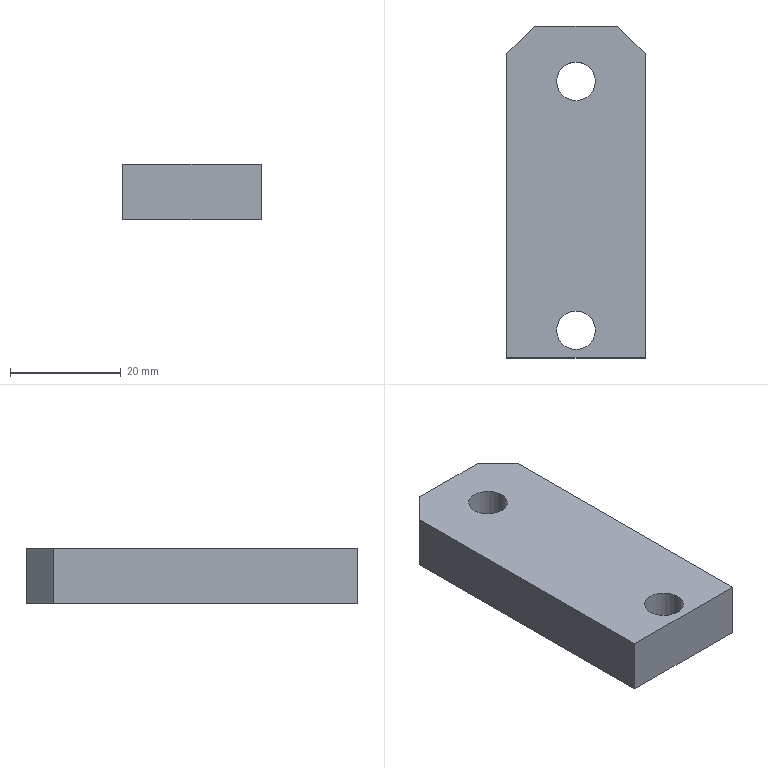Part | SolidWorks | features Chamfer 1, Extrusion 1, ICE 1 | 1 solid | 12 faces | box 25 x 60 x 10 mm | volume 13980 mm3 | plane 8 | cylinder 4 | commonest cylinder face diameters 7 x4
STEP:
#1=CARTESIAN_POINT('',(-3.5,20.,0.));
#2=VERTEX_POINT('',#1);
#3=CARTESIAN_POINT('',(3.5,20.,0.));
#4=VERTEX_POINT('',#3);
#5=CARTESIAN_POINT('',(0.,20.,0.));
#6=DIRECTION('',(0.,0.,1.));
#7=DIRECTION('',(1.,0.,0.));
#8=AXIS2_PLACEMENT_3D('',#5,#6,#7);
#9=CIRCLE('',#8,3.5);
#10=EDGE_CURVE('',#2,#4,#9,.T.);
#11=ORIENTED_EDGE('',*,*,#10,.F.);
#12=CARTESIAN_POINT('',(-3.5,20.,10.));
#13=VERTEX_POINT('',#12);
#14=CARTESIAN_POINT('',(-3.5,20.,0.));
#15=DIRECTION('',(0.,0.,1.));
#16=VECTOR('',#15,1000.);
#17=LINE('',#14,#16);
#18=EDGE_CURVE('',#2,#13,#17,.T.);
#19=ORIENTED_EDGE('',*,*,#18,.T.);
#20=CARTESIAN_POINT('',(3.5,20.,10.));
#21=VERTEX_POINT('',#20);
#22=CARTESIAN_POINT('',(0.,20.,10.));
#23=DIRECTION('',(0.,0.,1.));
#24=DIRECTION('',(1.,0.,0.));
#25=AXIS2_PLACEMENT_3D('',#22,#23,#24);
#26=CIRCLE('',#25,3.5);
#27=EDGE_CURVE('',#13,#21,#26,.T.);
#28=ORIENTED_EDGE('',*,*,#27,.T.);
#29=CARTESIAN_POINT('',(3.5,20.,0.));
#30=DIRECTION('',(0.,0.,1.));
#31=VECTOR('',#30,1000.);
#32=LINE('',#29,#31);
#33=EDGE_CURVE('',#4,#21,#32,.T.);
#34=ORIENTED_EDGE('',*,*,#33,.F.);
#35=EDGE_LOOP('',(#11,#19,#28,#34));
#36=FACE_OUTER_BOUND('',#35,.T.);
#37=CARTESIAN_POINT('',(0.,20.,0.));
#38=DIRECTION('',(0.,0.,1.));
#39=DIRECTION('',(1.,0.,0.));
#40=AXIS2_PLACEMENT_3D('',#37,#38,#39);
#41=CYLINDRICAL_SURFACE('',#40,3.5);
#42=ADVANCED_FACE('',(#36),#41,.F.);
#43=CARTESIAN_POINT('',(-3.5,-25.,0.));
#44=VERTEX_POINT('',#43);
#45=CARTESIAN_POINT('',(3.5,-25.,0.));
#46=VERTEX_POINT('',#45);
#47=CARTESIAN_POINT('',(0.,-25.,0.));
#48=DIRECTION('',(0.,0.,1.));
#49=DIRECTION('',(1.,0.,0.));
#50=AXIS2_PLACEMENT_3D('',#47,#48,#49);
#51=CIRCLE('',#50,3.5);
#52=EDGE_CURVE('',#44,#46,#51,.T.);
#53=ORIENTED_EDGE('',*,*,#52,.F.);
#54=CARTESIAN_POINT('',(-3.5,-25.,10.));
#55=VERTEX_POINT('',#54);
#56=CARTESIAN_POINT('',(-3.5,-25.,0.));
#57=DIRECTION('',(0.,0.,1.));
#58=VECTOR('',#57,1000.);
#59=LINE('',#56,#58);
#60=EDGE_CURVE('',#44,#55,#59,.T.);
#61=ORIENTED_EDGE('',*,*,#60,.T.);
#62=CARTESIAN_POINT('',(3.5,-25.,10.));
#63=VERTEX_POINT('',#62);
#64=CARTESIAN_POINT('',(0.,-25.,10.));
#65=DIRECTION('',(0.,0.,1.));
#66=DIRECTION('',(1.,0.,0.));
#67=AXIS2_PLACEMENT_3D('',#64,#65,#66);
#68=CIRCLE('',#67,3.5);
#69=EDGE_CURVE('',#55,#63,#68,.T.);
#70=ORIENTED_EDGE('',*,*,#69,.T.);
#71=CARTESIAN_POINT('',(3.5,-25.,0.));
#72=DIRECTION('',(0.,0.,1.));
#73=VECTOR('',#72,1000.);
#74=LINE('',#71,#73);
#75=EDGE_CURVE('',#46,#63,#74,.T.);
#76=ORIENTED_EDGE('',*,*,#75,.F.);
#77=EDGE_LOOP('',(#53,#61,#70,#76));
#78=FACE_OUTER_BOUND('',#77,.T.);
#79=CARTESIAN_POINT('',(0.,-25.,0.));
#80=DIRECTION('',(0.,0.,1.));
#81=DIRECTION('',(1.,0.,0.));
#82=AXIS2_PLACEMENT_3D('',#79,#80,#81);
#83=CYLINDRICAL_SURFACE('',#82,3.5);
#84=ADVANCED_FACE('',(#78),#83,.F.);
#85=CARTESIAN_POINT('',(-12.5,25.,10.));
#86=VERTEX_POINT('',#85);
#87=CARTESIAN_POINT('',(-12.5,-30.,10.));
#88=VERTEX_POINT('',#87);
#89=CARTESIAN_POINT('',(-12.5,30.,10.));
#90=DIRECTION('',(0.,-1.,0.));
#91=VECTOR('',#90,1000.);
#92=LINE('',#89,#91);
#93=EDGE_CURVE('',#86,#88,#92,.T.);
#94=ORIENTED_EDGE('',*,*,#93,.F.);
#95=CARTESIAN_POINT('',(-12.5,25.,0.));
#96=VERTEX_POINT('',#95);
#97=CARTESIAN_POINT('',(-12.5,25.,10.));
#98=DIRECTION('',(0.,0.,-1.));
#99=VECTOR('',#98,1000.);
#100=LINE('',#97,#99);
#101=EDGE_CURVE('',#86,#96,#100,.T.);
#102=ORIENTED_EDGE('',*,*,#101,.T.);
#103=CARTESIAN_POINT('',(-12.5,-30.,0.));
#104=VERTEX_POINT('',#103);
#105=CARTESIAN_POINT('',(-12.5,30.,0.));
#106=DIRECTION('',(0.,-1.,0.));
#107=VECTOR('',#106,1000.);
#108=LINE('',#105,#107);
#109=EDGE_CURVE('',#96,#104,#108,.T.);
#110=ORIENTED_EDGE('',*,*,#109,.T.);
#111=CARTESIAN_POINT('',(-12.5,-30.,10.));
#112=DIRECTION('',(0.,0.,-1.));
#113=VECTOR('',#112,1000.);
#114=LINE('',#111,#113);
#115=EDGE_CURVE('',#88,#104,#114,.T.);
#116=ORIENTED_EDGE('',*,*,#115,.F.);
#117=EDGE_LOOP('',(#94,#102,#110,#116));
#118=FACE_OUTER_BOUND('',#117,.T.);
#119=CARTESIAN_POINT('',(-12.5,30.,10.));
#120=DIRECTION('',(1.,0.,0.));
#121=DIRECTION('',(0.,1.,0.));
#122=AXIS2_PLACEMENT_3D('',#119,#120,#121);
#123=PLANE('',#122);
#124=ADVANCED_FACE('',(#118),#123,.F.);
#125=CARTESIAN_POINT('',(12.5,-30.,0.));
#126=VERTEX_POINT('',#125);
#127=CARTESIAN_POINT('',(12.5,-30.,0.));
#128=DIRECTION('',(1.,0.,0.));
#129=VECTOR('',#128,1000.);
#130=LINE('',#127,#129);
#131=EDGE_CURVE('',#104,#126,#130,.T.);
#132=ORIENTED_EDGE('',*,*,#131,.T.);
#133=CARTESIAN_POINT('',(12.5,-30.,10.));
#134=VERTEX_POINT('',#133);
#135=CARTESIAN_POINT('',(12.5,-30.,10.));
#136=DIRECTION('',(0.,0.,-1.));
#137=VECTOR('',#136,1000.);
#138=LINE('',#135,#137);
#139=EDGE_CURVE('',#134,#126,#138,.T.);
#140=ORIENTED_EDGE('',*,*,#139,.F.);
#141=CARTESIAN_POINT('',(12.5,-30.,10.));
#142=DIRECTION('',(1.,0.,0.));
#143=VECTOR('',#142,1000.);
#144=LINE('',#141,#143);
#145=EDGE_CURVE('',#88,#134,#144,.T.);
#146=ORIENTED_EDGE('',*,*,#145,.F.);
#147=ORIENTED_EDGE('',*,*,#115,.T.);
#148=EDGE_LOOP('',(#132,#140,#146,#147));
#149=FACE_OUTER_BOUND('',#148,.T.);
#150=CARTESIAN_POINT('',(12.5,-30.,10.));
#151=DIRECTION('',(0.,1.,0.));
#152=DIRECTION('',(-1.,0.,0.));
#153=AXIS2_PLACEMENT_3D('',#150,#151,#152);
#154=PLANE('',#153);
#155=ADVANCED_FACE('',(#149),#154,.F.);
#156=CARTESIAN_POINT('',(12.5,25.,0.));
#157=VERTEX_POINT('',#156);
#158=CARTESIAN_POINT('',(12.5,30.,0.));
#159=DIRECTION('',(0.,1.,0.));
#160=VECTOR('',#159,1000.);
#161=LINE('',#158,#160);
#162=EDGE_CURVE('',#126,#157,#161,.T.);
#163=ORIENTED_EDGE('',*,*,#162,.T.);
#164=CARTESIAN_POINT('',(12.5,25.,10.));
#165=VERTEX_POINT('',#164);
#166=CARTESIAN_POINT('',(12.5,25.,10.));
#167=DIRECTION('',(0.,0.,1.));
#168=VECTOR('',#167,1000.);
#169=LINE('',#166,#168);
#170=EDGE_CURVE('',#157,#165,#169,.T.);
#171=ORIENTED_EDGE('',*,*,#170,.T.);
#172=CARTESIAN_POINT('',(12.5,30.,10.));
#173=DIRECTION('',(0.,1.,0.));
#174=VECTOR('',#173,1000.);
#175=LINE('',#172,#174);
#176=EDGE_CURVE('',#134,#165,#175,.T.);
#177=ORIENTED_EDGE('',*,*,#176,.F.);
#178=ORIENTED_EDGE('',*,*,#139,.T.);
#179=EDGE_LOOP('',(#163,#171,#177,#178));
#180=FACE_OUTER_BOUND('',#179,.T.);
#181=CARTESIAN_POINT('',(12.5,30.,10.));
#182=DIRECTION('',(-1.,0.,0.));
#183=DIRECTION('',(0.,-1.,0.));
#184=AXIS2_PLACEMENT_3D('',#181,#182,#183);
#185=PLANE('',#184);
#186=ADVANCED_FACE('',(#180),#185,.F.);
#187=CARTESIAN_POINT('',(7.5,30.,10.));
#188=VERTEX_POINT('',#187);
#189=CARTESIAN_POINT('',(-7.5,30.,10.));
#190=VERTEX_POINT('',#189);
#191=CARTESIAN_POINT('',(12.5,30.,10.));
#192=DIRECTION('',(-1.,0.,0.));
#193=VECTOR('',#192,1000.);
#194=LINE('',#191,#193);
#195=EDGE_CURVE('',#188,#190,#194,.T.);
#196=ORIENTED_EDGE('',*,*,#195,.F.);
#197=CARTESIAN_POINT('',(7.5,30.,0.));
#198=VERTEX_POINT('',#197);
#199=CARTESIAN_POINT('',(7.5,30.,10.));
#200=DIRECTION('',(0.,0.,-1.));
#201=VECTOR('',#200,1000.);
#202=LINE('',#199,#201);
#203=EDGE_CURVE('',#188,#198,#202,.T.);
#204=ORIENTED_EDGE('',*,*,#203,.T.);
#205=CARTESIAN_POINT('',(-7.5,30.,0.));
#206=VERTEX_POINT('',#205);
#207=CARTESIAN_POINT('',(12.5,30.,0.));
#208=DIRECTION('',(-1.,0.,0.));
#209=VECTOR('',#208,1000.);
#210=LINE('',#207,#209);
#211=EDGE_CURVE('',#198,#206,#210,.T.);
#212=ORIENTED_EDGE('',*,*,#211,.T.);
#213=CARTESIAN_POINT('',(-7.5,30.,10.));
#214=DIRECTION('',(0.,0.,1.));
#215=VECTOR('',#214,1000.);
#216=LINE('',#213,#215);
#217=EDGE_CURVE('',#206,#190,#216,.T.);
#218=ORIENTED_EDGE('',*,*,#217,.T.);
#219=EDGE_LOOP('',(#196,#204,#212,#218));
#220=FACE_OUTER_BOUND('',#219,.T.);
#221=CARTESIAN_POINT('',(12.5,30.,10.));
#222=DIRECTION('',(0.,-1.,0.));
#223=DIRECTION('',(0.,0.,-1.));
#224=AXIS2_PLACEMENT_3D('',#221,#222,#223);
#225=PLANE('',#224);
#226=ADVANCED_FACE('',(#220),#225,.F.);
#227=CARTESIAN_POINT('',(0.,20.,10.));
#228=DIRECTION('',(0.,0.,1.));
#229=DIRECTION('',(1.,0.,0.));
#230=AXIS2_PLACEMENT_3D('',#227,#228,#229);
#231=CIRCLE('',#230,3.5);
#232=EDGE_CURVE('',#21,#13,#231,.T.);
#233=ORIENTED_EDGE('',*,*,#232,.F.);
#234=ORIENTED_EDGE('',*,*,#27,.F.);
#235=EDGE_LOOP('',(#233,#234));
#236=FACE_BOUND('',#235,.T.);
#237=CARTESIAN_POINT('',(0.,-25.,10.));
#238=DIRECTION('',(0.,0.,1.));
#239=DIRECTION('',(1.,0.,0.));
#240=AXIS2_PLACEMENT_3D('',#237,#238,#239);
#241=CIRCLE('',#240,3.5);
#242=EDGE_CURVE('',#63,#55,#241,.T.);
#243=ORIENTED_EDGE('',*,*,#242,.F.);
#244=ORIENTED_EDGE('',*,*,#69,.F.);
#245=EDGE_LOOP('',(#243,#244));
#246=FACE_BOUND('',#245,.T.);
#247=ORIENTED_EDGE('',*,*,#176,.T.);
#248=CARTESIAN_POINT('',(7.5,30.,10.));
#249=DIRECTION('',(-0.7071,0.7071,0.));
#250=VECTOR('',#249,1000.);
#251=LINE('',#248,#250);
#252=EDGE_CURVE('',#165,#188,#251,.T.);
#253=ORIENTED_EDGE('',*,*,#252,.T.);
#254=ORIENTED_EDGE('',*,*,#195,.T.);
#255=CARTESIAN_POINT('',(-12.5,25.,10.));
#256=DIRECTION('',(-0.7071,-0.7071,0.));
#257=VECTOR('',#256,1000.);
#258=LINE('',#255,#257);
#259=EDGE_CURVE('',#190,#86,#258,.T.);
#260=ORIENTED_EDGE('',*,*,#259,.T.);
#261=ORIENTED_EDGE('',*,*,#93,.T.);
#262=ORIENTED_EDGE('',*,*,#145,.T.);
#263=EDGE_LOOP('',(#247,#253,#254,#260,#261,#262));
#264=FACE_OUTER_BOUND('',#263,.T.);
#265=CARTESIAN_POINT('',(0.,0.,10.));
#266=DIRECTION('',(0.,0.,-1.));
#267=DIRECTION('',(-1.,0.,0.));
#268=AXIS2_PLACEMENT_3D('',#265,#266,#267);
#269=PLANE('',#268);
#270=ADVANCED_FACE('',(#236,#246,#264),#269,.F.);
#271=CARTESIAN_POINT('',(0.,20.,0.));
#272=DIRECTION('',(0.,0.,1.));
#273=DIRECTION('',(1.,0.,0.));
#274=AXIS2_PLACEMENT_3D('',#271,#272,#273);
#275=CIRCLE('',#274,3.5);
#276=EDGE_CURVE('',#4,#2,#275,.T.);
#277=ORIENTED_EDGE('',*,*,#276,.T.);
#278=ORIENTED_EDGE('',*,*,#10,.T.);
#279=EDGE_LOOP('',(#277,#278));
#280=FACE_BOUND('',#279,.T.);
#281=CARTESIAN_POINT('',(0.,-25.,0.));
#282=DIRECTION('',(0.,0.,1.));
#283=DIRECTION('',(1.,0.,0.));
#284=AXIS2_PLACEMENT_3D('',#281,#282,#283);
#285=CIRCLE('',#284,3.5);
#286=EDGE_CURVE('',#46,#44,#285,.T.);
#287=ORIENTED_EDGE('',*,*,#286,.T.);
#288=ORIENTED_EDGE('',*,*,#52,.T.);
#289=EDGE_LOOP('',(#287,#288));
#290=FACE_BOUND('',#289,.T.);
#291=ORIENTED_EDGE('',*,*,#211,.F.);
#292=CARTESIAN_POINT('',(18.75,18.75,0.));
#293=DIRECTION('',(0.7071,-0.7071,0.));
#294=VECTOR('',#293,1000.);
#295=LINE('',#292,#294);
#296=EDGE_CURVE('',#198,#157,#295,.T.);
#297=ORIENTED_EDGE('',*,*,#296,.T.);
#298=ORIENTED_EDGE('',*,*,#162,.F.);
#299=ORIENTED_EDGE('',*,*,#131,.F.);
#300=ORIENTED_EDGE('',*,*,#109,.F.);
#301=CARTESIAN_POINT('',(-18.75,18.75,0.));
#302=DIRECTION('',(0.7071,0.7071,0.));
#303=VECTOR('',#302,1000.);
#304=LINE('',#301,#303);
#305=EDGE_CURVE('',#96,#206,#304,.T.);
#306=ORIENTED_EDGE('',*,*,#305,.T.);
#307=EDGE_LOOP('',(#291,#297,#298,#299,#300,#306));
#308=FACE_OUTER_BOUND('',#307,.T.);
#309=CARTESIAN_POINT('',(0.,0.,0.));
#310=DIRECTION('',(0.,0.,-1.));
#311=DIRECTION('',(-1.,0.,0.));
#312=AXIS2_PLACEMENT_3D('',#309,#310,#311);
#313=PLANE('',#312);
#314=ADVANCED_FACE('',(#280,#290,#308),#313,.T.);
#315=ORIENTED_EDGE('',*,*,#60,.F.);
#316=ORIENTED_EDGE('',*,*,#286,.F.);
#317=ORIENTED_EDGE('',*,*,#75,.T.);
#318=ORIENTED_EDGE('',*,*,#242,.T.);
#319=EDGE_LOOP('',(#315,#316,#317,#318));
#320=FACE_OUTER_BOUND('',#319,.T.);
#321=CARTESIAN_POINT('',(0.,-25.,0.));
#322=DIRECTION('',(0.,0.,1.));
#323=DIRECTION('',(1.,0.,0.));
#324=AXIS2_PLACEMENT_3D('',#321,#322,#323);
#325=CYLINDRICAL_SURFACE('',#324,3.5);
#326=ADVANCED_FACE('',(#320),#325,.F.);
#327=ORIENTED_EDGE('',*,*,#18,.F.);
#328=ORIENTED_EDGE('',*,*,#276,.F.);
#329=ORIENTED_EDGE('',*,*,#33,.T.);
#330=ORIENTED_EDGE('',*,*,#232,.T.);
#331=EDGE_LOOP('',(#327,#328,#329,#330));
#332=FACE_OUTER_BOUND('',#331,.T.);
#333=CARTESIAN_POINT('',(0.,20.,0.));
#334=DIRECTION('',(0.,0.,1.));
#335=DIRECTION('',(1.,0.,0.));
#336=AXIS2_PLACEMENT_3D('',#333,#334,#335);
#337=CYLINDRICAL_SURFACE('',#336,3.5);
#338=ADVANCED_FACE('',(#332),#337,.F.);
#339=ORIENTED_EDGE('',*,*,#252,.F.);
#340=ORIENTED_EDGE('',*,*,#170,.F.);
#341=ORIENTED_EDGE('',*,*,#296,.F.);
#342=ORIENTED_EDGE('',*,*,#203,.F.);
#343=EDGE_LOOP('',(#339,#340,#341,#342));
#344=FACE_OUTER_BOUND('',#343,.T.);
#345=CARTESIAN_POINT('',(7.5,30.,10.));
#346=DIRECTION('',(-0.7071,-0.7071,0.));
#347=DIRECTION('',(0.,0.,-1.));
#348=AXIS2_PLACEMENT_3D('',#345,#346,#347);
#349=PLANE('',#348);
#350=ADVANCED_FACE('',(#344),#349,.F.);
#351=ORIENTED_EDGE('',*,*,#259,.F.);
#352=ORIENTED_EDGE('',*,*,#217,.F.);
#353=ORIENTED_EDGE('',*,*,#305,.F.);
#354=ORIENTED_EDGE('',*,*,#101,.F.);
#355=EDGE_LOOP('',(#351,#352,#353,#354));
#356=FACE_OUTER_BOUND('',#355,.T.);
#357=CARTESIAN_POINT('',(-12.5,25.,10.));
#358=DIRECTION('',(0.7071,-0.7071,0.));
#359=DIRECTION('',(0.,0.,-1.));
#360=AXIS2_PLACEMENT_3D('',#357,#358,#359);
#361=PLANE('',#360);
#362=ADVANCED_FACE('',(#356),#361,.F.);
#363=CLOSED_SHELL('',(#42,#84,#124,#155,#186,#226,#270,#314,#326,#338,#350,#362));
#364=MANIFOLD_SOLID_BREP('',#363);
#365=CARTESIAN_POINT('',(0.,0.,0.));
#366=DIRECTION('',(0.,0.,1.));
#367=DIRECTION('',(1.,0.,0.));
#368=AXIS2_PLACEMENT_3D('',#365,#366,#367);
#369=(LENGTH_UNIT()NAMED_UNIT(*)SI_UNIT(.MILLI.,.METRE.));
#370=UNCERTAINTY_MEASURE_WITH_UNIT(LENGTH_MEASURE(0.00001),#369,'','');
#371=(NAMED_UNIT(*)PLANE_ANGLE_UNIT()SI_UNIT($,.RADIAN.));
#372=(NAMED_UNIT(*)SI_UNIT($,.STERADIAN.)SOLID_ANGLE_UNIT());
#373=(GEOMETRIC_REPRESENTATION_CONTEXT(3)GLOBAL_UNCERTAINTY_ASSIGNED_CONTEXT((#370))GLOBAL_UNIT_ASSIGNED_CONTEXT((#369,#371,#372))REPRESENTATION_CONTEXT('',''));
#374=ADVANCED_BREP_SHAPE_REPRESENTATION('',(#364,#368),#373);